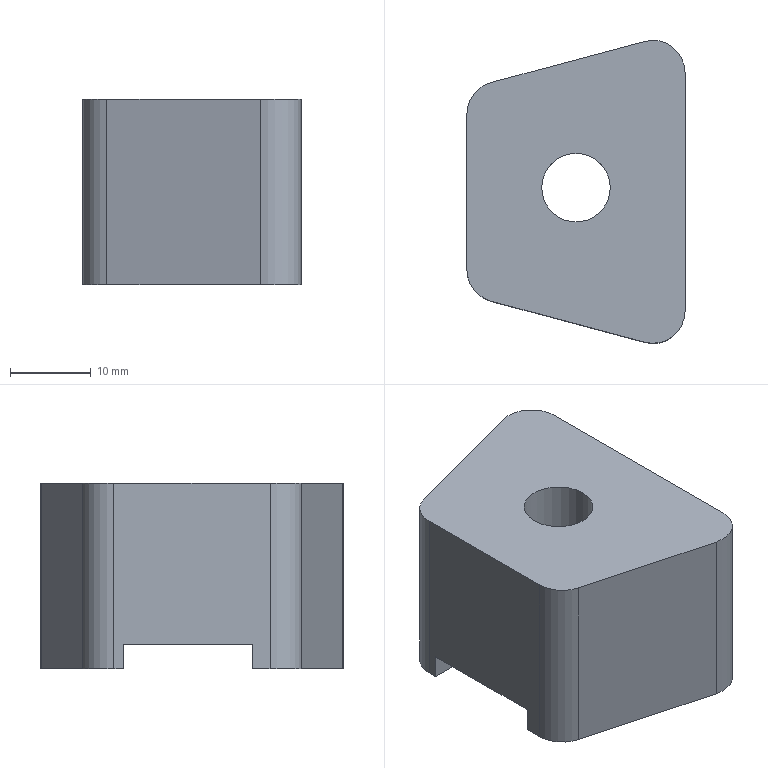Part | NX | features solid 2 | 1 solid | 17 faces | box 27 x 37.502 x 23 mm | volume 16532 mm3 | plane 11 | cylinder 6 | commonest cylinder face diameters 8 x4 8.5 x1 14 x1
STEP:
#1=CARTESIAN_POINT('',(1429.324,0.,20.));
#2=VERTEX_POINT('',#1);
#3=CARTESIAN_POINT('',(1425.074,0.,20.));
#4=DIRECTION('',(0.,0.,1.));
#5=DIRECTION('',(1.,0.,0.));
#6=AXIS2_PLACEMENT_3D('',#3,#4,#5);
#7=CIRCLE('',#6,4.25);
#8=EDGE_CURVE('',#2,#2,#7,.T.);
#9=ORIENTED_EDGE('',*,*,#8,.F.);
#10=EDGE_LOOP('',(#9));
#11=FACE_BOUND('',#10,.T.);
#12=CARTESIAN_POINT('',(1414.539,-14.041,20.));
#13=VERTEX_POINT('',#12);
#14=CARTESIAN_POINT('',(1433.539,-19.132,20.));
#15=VERTEX_POINT('',#14);
#16=CARTESIAN_POINT('',(1515.869,-41.192,20.));
#17=DIRECTION('',(0.9659,-0.2588,0.));
#18=VECTOR('',#17,1000.);
#19=LINE('',#16,#18);
#20=EDGE_CURVE('',#13,#15,#19,.T.);
#21=ORIENTED_EDGE('',*,*,#20,.T.);
#22=CARTESIAN_POINT('',(1438.574,-15.268,20.));
#23=VERTEX_POINT('',#22);
#24=CARTESIAN_POINT('',(1434.574,-15.268,20.));
#25=DIRECTION('',(0.,0.,1.));
#26=DIRECTION('',(1.,0.,0.));
#27=AXIS2_PLACEMENT_3D('',#24,#25,#26);
#28=CIRCLE('',#27,4.);
#29=EDGE_CURVE('',#15,#23,#28,.T.);
#30=ORIENTED_EDGE('',*,*,#29,.T.);
#31=CARTESIAN_POINT('',(1438.574,14.233,20.));
#32=VERTEX_POINT('',#31);
#33=CARTESIAN_POINT('',(1438.574,-11.19,20.));
#34=DIRECTION('',(0.,-1.,0.));
#35=VECTOR('',#34,1000.);
#36=LINE('',#33,#35);
#37=EDGE_CURVE('',#32,#23,#36,.T.);
#38=ORIENTED_EDGE('',*,*,#37,.F.);
#39=CARTESIAN_POINT('',(1433.539,18.097,20.));
#40=VERTEX_POINT('',#39);
#41=CARTESIAN_POINT('',(1434.574,14.233,20.));
#42=DIRECTION('',(0.,0.,1.));
#43=DIRECTION('',(1.,0.,0.));
#44=AXIS2_PLACEMENT_3D('',#41,#42,#43);
#45=CIRCLE('',#44,4.);
#46=EDGE_CURVE('',#32,#40,#45,.T.);
#47=ORIENTED_EDGE('',*,*,#46,.T.);
#48=CARTESIAN_POINT('',(1414.539,13.006,20.));
#49=VERTEX_POINT('',#48);
#50=CARTESIAN_POINT('',(1460.853,25.416,20.));
#51=DIRECTION('',(-0.9659,-0.2588,0.));
#52=VECTOR('',#51,1000.);
#53=LINE('',#50,#52);
#54=EDGE_CURVE('',#40,#49,#53,.T.);
#55=ORIENTED_EDGE('',*,*,#54,.T.);
#56=CARTESIAN_POINT('',(1411.574,9.142,20.));
#57=VERTEX_POINT('',#56);
#58=CARTESIAN_POINT('',(1415.574,9.142,20.));
#59=DIRECTION('',(0.,0.,1.));
#60=DIRECTION('',(1.,0.,0.));
#61=AXIS2_PLACEMENT_3D('',#58,#59,#60);
#62=CIRCLE('',#61,4.);
#63=EDGE_CURVE('',#49,#57,#62,.T.);
#64=ORIENTED_EDGE('',*,*,#63,.T.);
#65=CARTESIAN_POINT('',(1411.574,-10.177,20.));
#66=VERTEX_POINT('',#65);
#67=CARTESIAN_POINT('',(1411.574,-7.,20.));
#68=DIRECTION('',(0.,1.,0.));
#69=VECTOR('',#68,1000.);
#70=LINE('',#67,#69);
#71=EDGE_CURVE('',#66,#57,#70,.T.);
#72=ORIENTED_EDGE('',*,*,#71,.F.);
#73=CARTESIAN_POINT('',(1415.574,-10.177,20.));
#74=DIRECTION('',(0.,0.,1.));
#75=DIRECTION('',(1.,0.,0.));
#76=AXIS2_PLACEMENT_3D('',#73,#74,#75);
#77=CIRCLE('',#76,4.);
#78=EDGE_CURVE('',#66,#13,#77,.T.);
#79=ORIENTED_EDGE('',*,*,#78,.T.);
#80=EDGE_LOOP('',(#21,#30,#38,#47,#55,#64,#72,#79));
#81=FACE_BOUND('',#80,.T.);
#82=CARTESIAN_POINT('',(1497.285,-110.548,20.));
#83=DIRECTION('',(0.,0.,1.));
#84=DIRECTION('',(1.,0.,0.));
#85=AXIS2_PLACEMENT_3D('',#82,#83,#84);
#86=PLANE('',#85);
#87=ADVANCED_FACE('',(#11,#81),#86,.T.);
#88=CARTESIAN_POINT('',(1438.574,-8.,0.));
#89=VERTEX_POINT('',#88);
#90=CARTESIAN_POINT('',(1411.574,-8.,0.));
#91=VERTEX_POINT('',#90);
#92=CARTESIAN_POINT('',(1423.85,-8.,0.));
#93=DIRECTION('',(-1.,0.,0.));
#94=VECTOR('',#93,1000.);
#95=LINE('',#92,#94);
#96=EDGE_CURVE('',#89,#91,#95,.T.);
#97=ORIENTED_EDGE('',*,*,#96,.F.);
#98=CARTESIAN_POINT('',(1438.574,-8.,-3.));
#99=VERTEX_POINT('',#98);
#100=CARTESIAN_POINT('',(1438.574,-8.,-5.));
#101=DIRECTION('',(0.,0.,1.));
#102=VECTOR('',#101,1000.);
#103=LINE('',#100,#102);
#104=EDGE_CURVE('',#99,#89,#103,.T.);
#105=ORIENTED_EDGE('',*,*,#104,.F.);
#106=CARTESIAN_POINT('',(1411.574,-8.,-3.));
#107=VERTEX_POINT('',#106);
#108=CARTESIAN_POINT('',(268.879,-8.,-3.));
#109=DIRECTION('',(-1.,0.,0.));
#110=VECTOR('',#109,1000.);
#111=LINE('',#108,#110);
#112=EDGE_CURVE('',#107,#99,#111,.F.);
#113=ORIENTED_EDGE('',*,*,#112,.F.);
#114=CARTESIAN_POINT('',(1411.574,-8.,-5.));
#115=DIRECTION('',(0.,0.,1.));
#116=VECTOR('',#115,1000.);
#117=LINE('',#114,#116);
#118=EDGE_CURVE('',#107,#91,#117,.T.);
#119=ORIENTED_EDGE('',*,*,#118,.T.);
#120=EDGE_LOOP('',(#97,#105,#113,#119));
#121=FACE_BOUND('',#120,.T.);
#122=CARTESIAN_POINT('',(1423.85,-8.,-5.));
#123=DIRECTION('',(0.,1.,0.));
#124=DIRECTION('',(0.,0.,-1.));
#125=AXIS2_PLACEMENT_3D('',#122,#123,#124);
#126=PLANE('',#125);
#127=ADVANCED_FACE('',(#121),#126,.T.);
#128=CARTESIAN_POINT('',(1438.574,-15.268,-3.));
#129=VERTEX_POINT('',#128);
#130=CARTESIAN_POINT('',(1438.574,0.,-3.));
#131=DIRECTION('',(0.,1.,0.));
#132=VECTOR('',#131,1000.);
#133=LINE('',#130,#132);
#134=EDGE_CURVE('',#99,#129,#133,.F.);
#135=ORIENTED_EDGE('',*,*,#134,.T.);
#136=CARTESIAN_POINT('',(1433.539,-19.132,-3.));
#137=VERTEX_POINT('',#136);
#138=CARTESIAN_POINT('',(1434.574,-15.268,-3.));
#139=DIRECTION('',(0.,0.,1.));
#140=DIRECTION('',(1.,0.,0.));
#141=AXIS2_PLACEMENT_3D('',#138,#139,#140);
#142=CIRCLE('',#141,4.);
#143=EDGE_CURVE('',#129,#137,#142,.F.);
#144=ORIENTED_EDGE('',*,*,#143,.T.);
#145=CARTESIAN_POINT('',(1414.539,-14.041,-3.));
#146=VERTEX_POINT('',#145);
#147=CARTESIAN_POINT('',(1417.086,-14.724,-3.));
#148=DIRECTION('',(-0.9659,0.2588,0.));
#149=VECTOR('',#148,1000.);
#150=LINE('',#147,#149);
#151=EDGE_CURVE('',#146,#137,#150,.F.);
#152=ORIENTED_EDGE('',*,*,#151,.F.);
#153=CARTESIAN_POINT('',(1411.574,-10.177,-3.));
#154=VERTEX_POINT('',#153);
#155=CARTESIAN_POINT('',(1415.574,-10.177,-3.));
#156=DIRECTION('',(0.,0.,1.));
#157=DIRECTION('',(1.,0.,0.));
#158=AXIS2_PLACEMENT_3D('',#155,#156,#157);
#159=CIRCLE('',#158,4.);
#160=EDGE_CURVE('',#146,#154,#159,.F.);
#161=ORIENTED_EDGE('',*,*,#160,.T.);
#162=CARTESIAN_POINT('',(1411.574,0.,-3.));
#163=DIRECTION('',(0.,-1.,0.));
#164=VECTOR('',#163,1000.);
#165=LINE('',#162,#164);
#166=EDGE_CURVE('',#154,#107,#165,.F.);
#167=ORIENTED_EDGE('',*,*,#166,.T.);
#168=ORIENTED_EDGE('',*,*,#112,.T.);
#169=EDGE_LOOP('',(#135,#144,#152,#161,#167,#168));
#170=FACE_BOUND('',#169,.T.);
#171=CARTESIAN_POINT('',(268.879,0.,-3.));
#172=DIRECTION('',(0.,0.,1.));
#173=DIRECTION('',(1.,0.,0.));
#174=AXIS2_PLACEMENT_3D('',#171,#172,#173);
#175=PLANE('',#174);
#176=ADVANCED_FACE('',(#170),#175,.F.);
#177=ORIENTED_EDGE('',*,*,#151,.T.);
#178=CARTESIAN_POINT('',(1433.539,-19.132,-16.4));
#179=DIRECTION('',(0.,0.,-1.));
#180=VECTOR('',#179,1000.);
#181=LINE('',#178,#180);
#182=EDGE_CURVE('',#137,#15,#181,.F.);
#183=ORIENTED_EDGE('',*,*,#182,.T.);
#184=ORIENTED_EDGE('',*,*,#20,.F.);
#185=CARTESIAN_POINT('',(1414.539,-14.041,-16.4));
#186=DIRECTION('',(0.,0.,1.));
#187=VECTOR('',#186,1000.);
#188=LINE('',#185,#187);
#189=EDGE_CURVE('',#13,#146,#188,.F.);
#190=ORIENTED_EDGE('',*,*,#189,.T.);
#191=EDGE_LOOP('',(#177,#183,#184,#190));
#192=FACE_BOUND('',#191,.T.);
#193=CARTESIAN_POINT('',(1417.086,-14.724,-16.4));
#194=DIRECTION('',(-0.2588,-0.9659,0.));
#195=DIRECTION('',(-0.9659,0.2588,0.));
#196=AXIS2_PLACEMENT_3D('',#193,#194,#195);
#197=PLANE('',#196);
#198=ADVANCED_FACE('',(#192),#197,.T.);
#199=ORIENTED_EDGE('',*,*,#37,.T.);
#200=CARTESIAN_POINT('',(1438.574,-15.268,-5.));
#201=DIRECTION('',(0.,0.,-1.));
#202=VECTOR('',#201,1000.);
#203=LINE('',#200,#202);
#204=EDGE_CURVE('',#23,#129,#203,.T.);
#205=ORIENTED_EDGE('',*,*,#204,.T.);
#206=ORIENTED_EDGE('',*,*,#134,.F.);
#207=ORIENTED_EDGE('',*,*,#104,.T.);
#208=CARTESIAN_POINT('',(1438.574,8.,0.));
#209=VERTEX_POINT('',#208);
#210=CARTESIAN_POINT('',(1438.574,1232.968,0.));
#211=DIRECTION('',(0.,-1.,0.));
#212=VECTOR('',#211,1000.);
#213=LINE('',#210,#212);
#214=EDGE_CURVE('',#209,#89,#213,.T.);
#215=ORIENTED_EDGE('',*,*,#214,.F.);
#216=CARTESIAN_POINT('',(1438.574,8.,-3.));
#217=VERTEX_POINT('',#216);
#218=CARTESIAN_POINT('',(1438.574,8.,-5.));
#219=DIRECTION('',(0.,0.,1.));
#220=VECTOR('',#219,1000.);
#221=LINE('',#218,#220);
#222=EDGE_CURVE('',#217,#209,#221,.T.);
#223=ORIENTED_EDGE('',*,*,#222,.F.);
#224=CARTESIAN_POINT('',(1438.574,14.233,-3.));
#225=VERTEX_POINT('',#224);
#226=CARTESIAN_POINT('',(1438.574,-11.19,-3.));
#227=DIRECTION('',(0.,-1.,0.));
#228=VECTOR('',#227,1000.);
#229=LINE('',#226,#228);
#230=EDGE_CURVE('',#217,#225,#229,.F.);
#231=ORIENTED_EDGE('',*,*,#230,.T.);
#232=CARTESIAN_POINT('',(1438.574,14.233,-5.));
#233=DIRECTION('',(0.,0.,1.));
#234=VECTOR('',#233,1000.);
#235=LINE('',#232,#234);
#236=EDGE_CURVE('',#225,#32,#235,.T.);
#237=ORIENTED_EDGE('',*,*,#236,.T.);
#238=EDGE_LOOP('',(#199,#205,#206,#207,#215,#223,#231,#237));
#239=FACE_BOUND('',#238,.T.);
#240=CARTESIAN_POINT('',(1438.574,-11.19,-5.));
#241=DIRECTION('',(1.,0.,0.));
#242=DIRECTION('',(0.,0.,-1.));
#243=AXIS2_PLACEMENT_3D('',#240,#241,#242);
#244=PLANE('',#243);
#245=ADVANCED_FACE('',(#239),#244,.T.);
#246=ORIENTED_EDGE('',*,*,#166,.F.);
#247=CARTESIAN_POINT('',(1411.574,-10.177,-5.));
#248=DIRECTION('',(0.,0.,1.));
#249=VECTOR('',#248,1000.);
#250=LINE('',#247,#249);
#251=EDGE_CURVE('',#154,#66,#250,.T.);
#252=ORIENTED_EDGE('',*,*,#251,.T.);
#253=ORIENTED_EDGE('',*,*,#71,.T.);
#254=CARTESIAN_POINT('',(1411.574,9.142,-3.));
#255=VERTEX_POINT('',#254);
#256=CARTESIAN_POINT('',(1411.574,9.142,-5.));
#257=DIRECTION('',(0.,0.,-1.));
#258=VECTOR('',#257,1000.);
#259=LINE('',#256,#258);
#260=EDGE_CURVE('',#57,#255,#259,.T.);
#261=ORIENTED_EDGE('',*,*,#260,.T.);
#262=CARTESIAN_POINT('',(1411.574,8.,-3.));
#263=VERTEX_POINT('',#262);
#264=CARTESIAN_POINT('',(1411.574,0.,-3.));
#265=DIRECTION('',(0.,-1.,0.));
#266=VECTOR('',#265,1000.);
#267=LINE('',#264,#266);
#268=EDGE_CURVE('',#263,#255,#267,.F.);
#269=ORIENTED_EDGE('',*,*,#268,.F.);
#270=CARTESIAN_POINT('',(1411.574,8.,0.));
#271=VERTEX_POINT('',#270);
#272=CARTESIAN_POINT('',(1411.574,8.,-5.));
#273=DIRECTION('',(0.,0.,-1.));
#274=VECTOR('',#273,1000.);
#275=LINE('',#272,#274);
#276=EDGE_CURVE('',#271,#263,#275,.T.);
#277=ORIENTED_EDGE('',*,*,#276,.F.);
#278=CARTESIAN_POINT('',(1411.574,1232.968,0.));
#279=DIRECTION('',(0.,1.,0.));
#280=VECTOR('',#279,1000.);
#281=LINE('',#278,#280);
#282=EDGE_CURVE('',#91,#271,#281,.T.);
#283=ORIENTED_EDGE('',*,*,#282,.F.);
#284=ORIENTED_EDGE('',*,*,#118,.F.);
#285=EDGE_LOOP('',(#246,#252,#253,#261,#269,#277,#283,#284));
#286=FACE_BOUND('',#285,.T.);
#287=CARTESIAN_POINT('',(1411.574,-7.,-5.));
#288=DIRECTION('',(-1.,0.,0.));
#289=DIRECTION('',(0.,0.,1.));
#290=AXIS2_PLACEMENT_3D('',#287,#288,#289);
#291=PLANE('',#290);
#292=ADVANCED_FACE('',(#286),#291,.T.);
#293=CARTESIAN_POINT('',(1423.85,8.,0.));
#294=DIRECTION('',(1.,0.,0.));
#295=VECTOR('',#294,1000.);
#296=LINE('',#293,#295);
#297=EDGE_CURVE('',#271,#209,#296,.T.);
#298=ORIENTED_EDGE('',*,*,#297,.F.);
#299=ORIENTED_EDGE('',*,*,#276,.T.);
#300=CARTESIAN_POINT('',(1423.85,8.,-3.));
#301=DIRECTION('',(-1.,0.,0.));
#302=VECTOR('',#301,1000.);
#303=LINE('',#300,#302);
#304=EDGE_CURVE('',#263,#217,#303,.F.);
#305=ORIENTED_EDGE('',*,*,#304,.T.);
#306=ORIENTED_EDGE('',*,*,#222,.T.);
#307=EDGE_LOOP('',(#298,#299,#305,#306));
#308=FACE_BOUND('',#307,.T.);
#309=CARTESIAN_POINT('',(1423.85,8.,-5.));
#310=DIRECTION('',(0.,-1.,0.));
#311=DIRECTION('',(0.,0.,-1.));
#312=AXIS2_PLACEMENT_3D('',#309,#310,#311);
#313=PLANE('',#312);
#314=ADVANCED_FACE('',(#308),#313,.T.);
#315=CARTESIAN_POINT('',(1414.539,13.006,-3.));
#316=VERTEX_POINT('',#315);
#317=CARTESIAN_POINT('',(1433.539,18.097,-3.));
#318=VERTEX_POINT('',#317);
#319=CARTESIAN_POINT('',(342.372,-274.28,-3.));
#320=DIRECTION('',(-0.9659,-0.2588,0.));
#321=VECTOR('',#320,1000.);
#322=LINE('',#319,#321);
#323=EDGE_CURVE('',#316,#318,#322,.F.);
#324=ORIENTED_EDGE('',*,*,#323,.T.);
#325=CARTESIAN_POINT('',(1434.574,14.233,-3.));
#326=DIRECTION('',(0.,0.,1.));
#327=DIRECTION('',(1.,0.,0.));
#328=AXIS2_PLACEMENT_3D('',#325,#326,#327);
#329=CIRCLE('',#328,4.);
#330=EDGE_CURVE('',#318,#225,#329,.F.);
#331=ORIENTED_EDGE('',*,*,#330,.T.);
#332=ORIENTED_EDGE('',*,*,#230,.F.);
#333=ORIENTED_EDGE('',*,*,#304,.F.);
#334=ORIENTED_EDGE('',*,*,#268,.T.);
#335=CARTESIAN_POINT('',(1415.574,9.142,-3.));
#336=DIRECTION('',(0.,0.,1.));
#337=DIRECTION('',(1.,0.,0.));
#338=AXIS2_PLACEMENT_3D('',#335,#336,#337);
#339=CIRCLE('',#338,4.);
#340=EDGE_CURVE('',#255,#316,#339,.F.);
#341=ORIENTED_EDGE('',*,*,#340,.T.);
#342=EDGE_LOOP('',(#324,#331,#332,#333,#334,#341));
#343=FACE_BOUND('',#342,.T.);
#344=CARTESIAN_POINT('',(268.879,0.,-3.));
#345=DIRECTION('',(0.,0.,1.));
#346=DIRECTION('',(1.,0.,0.));
#347=AXIS2_PLACEMENT_3D('',#344,#345,#346);
#348=PLANE('',#347);
#349=ADVANCED_FACE('',(#343),#348,.F.);
#350=ORIENTED_EDGE('',*,*,#54,.F.);
#351=CARTESIAN_POINT('',(1433.539,18.097,-16.4));
#352=DIRECTION('',(0.,0.,1.));
#353=VECTOR('',#352,1000.);
#354=LINE('',#351,#353);
#355=EDGE_CURVE('',#40,#318,#354,.F.);
#356=ORIENTED_EDGE('',*,*,#355,.T.);
#357=ORIENTED_EDGE('',*,*,#323,.F.);
#358=CARTESIAN_POINT('',(1414.539,13.006,-16.4));
#359=DIRECTION('',(0.,0.,-1.));
#360=VECTOR('',#359,1000.);
#361=LINE('',#358,#360);
#362=EDGE_CURVE('',#316,#49,#361,.F.);
#363=ORIENTED_EDGE('',*,*,#362,.T.);
#364=EDGE_LOOP('',(#350,#356,#357,#363));
#365=FACE_BOUND('',#364,.T.);
#366=CARTESIAN_POINT('',(1417.345,13.758,-16.4));
#367=DIRECTION('',(-0.2588,0.9659,0.));
#368=DIRECTION('',(-0.9659,-0.2588,0.));
#369=AXIS2_PLACEMENT_3D('',#366,#367,#368);
#370=PLANE('',#369);
#371=ADVANCED_FACE('',(#365),#370,.T.);
#372=ORIENTED_EDGE('',*,*,#297,.T.);
#373=ORIENTED_EDGE('',*,*,#214,.T.);
#374=ORIENTED_EDGE('',*,*,#96,.T.);
#375=ORIENTED_EDGE('',*,*,#282,.T.);
#376=EDGE_LOOP('',(#372,#373,#374,#375));
#377=FACE_BOUND('',#376,.T.);
#378=CARTESIAN_POINT('',(1418.074,0.,0.));
#379=VERTEX_POINT('',#378);
#380=CARTESIAN_POINT('',(1425.074,0.,0.));
#381=DIRECTION('',(0.,0.,-1.));
#382=DIRECTION('',(-1.,0.,0.));
#383=AXIS2_PLACEMENT_3D('',#380,#381,#382);
#384=CIRCLE('',#383,7.);
#385=EDGE_CURVE('',#379,#379,#384,.F.);
#386=ORIENTED_EDGE('',*,*,#385,.T.);
#387=EDGE_LOOP('',(#386));
#388=FACE_BOUND('',#387,.T.);
#389=CARTESIAN_POINT('',(476.557,1232.968,0.));
#390=DIRECTION('',(0.,0.,-1.));
#391=DIRECTION('',(-0.9659,0.2588,0.));
#392=AXIS2_PLACEMENT_3D('',#389,#390,#391);
#393=PLANE('',#392);
#394=ADVANCED_FACE('',(#377,#388),#393,.T.);
#395=ORIENTED_EDGE('',*,*,#78,.F.);
#396=ORIENTED_EDGE('',*,*,#251,.F.);
#397=ORIENTED_EDGE('',*,*,#160,.F.);
#398=ORIENTED_EDGE('',*,*,#189,.F.);
#399=EDGE_LOOP('',(#395,#396,#397,#398));
#400=FACE_BOUND('',#399,.T.);
#401=CARTESIAN_POINT('',(1415.574,-10.177,-5.));
#402=DIRECTION('',(0.,0.,1.));
#403=DIRECTION('',(1.,0.,0.));
#404=AXIS2_PLACEMENT_3D('',#401,#402,#403);
#405=CYLINDRICAL_SURFACE('',#404,4.);
#406=ADVANCED_FACE('',(#400),#405,.T.);
#407=ORIENTED_EDGE('',*,*,#340,.F.);
#408=ORIENTED_EDGE('',*,*,#260,.F.);
#409=ORIENTED_EDGE('',*,*,#63,.F.);
#410=ORIENTED_EDGE('',*,*,#362,.F.);
#411=EDGE_LOOP('',(#407,#408,#409,#410));
#412=FACE_BOUND('',#411,.T.);
#413=CARTESIAN_POINT('',(1415.574,9.142,-5.));
#414=DIRECTION('',(0.,0.,-1.));
#415=DIRECTION('',(-1.,0.,0.));
#416=AXIS2_PLACEMENT_3D('',#413,#414,#415);
#417=CYLINDRICAL_SURFACE('',#416,4.);
#418=ADVANCED_FACE('',(#412),#417,.T.);
#419=ORIENTED_EDGE('',*,*,#8,.T.);
#420=EDGE_LOOP('',(#419));
#421=FACE_BOUND('',#420,.T.);
#422=CARTESIAN_POINT('',(1429.324,0.,10.));
#423=VERTEX_POINT('',#422);
#424=CARTESIAN_POINT('',(1425.074,0.,10.));
#425=DIRECTION('',(0.,0.,1.));
#426=DIRECTION('',(1.,0.,0.));
#427=AXIS2_PLACEMENT_3D('',#424,#425,#426);
#428=CIRCLE('',#427,4.25);
#429=EDGE_CURVE('',#423,#423,#428,.F.);
#430=ORIENTED_EDGE('',*,*,#429,.T.);
#431=EDGE_LOOP('',(#430));
#432=FACE_BOUND('',#431,.T.);
#433=CARTESIAN_POINT('',(1425.074,0.,50.));
#434=DIRECTION('',(0.,0.,1.));
#435=DIRECTION('',(1.,0.,0.));
#436=AXIS2_PLACEMENT_3D('',#433,#434,#435);
#437=CYLINDRICAL_SURFACE('',#436,4.25);
#438=ADVANCED_FACE('',(#421,#432),#437,.F.);
#439=ORIENTED_EDGE('',*,*,#429,.F.);
#440=EDGE_LOOP('',(#439));
#441=FACE_BOUND('',#440,.T.);
#442=CARTESIAN_POINT('',(1432.074,0.,10.));
#443=VERTEX_POINT('',#442);
#444=CARTESIAN_POINT('',(1425.074,0.,10.));
#445=DIRECTION('',(0.,0.,1.));
#446=DIRECTION('',(1.,0.,0.));
#447=AXIS2_PLACEMENT_3D('',#444,#445,#446);
#448=CIRCLE('',#447,7.);
#449=EDGE_CURVE('',#443,#443,#448,.F.);
#450=ORIENTED_EDGE('',*,*,#449,.T.);
#451=EDGE_LOOP('',(#450));
#452=FACE_BOUND('',#451,.T.);
#453=CARTESIAN_POINT('',(1425.074,0.,10.));
#454=DIRECTION('',(0.,0.,1.));
#455=DIRECTION('',(1.,0.,0.));
#456=AXIS2_PLACEMENT_3D('',#453,#454,#455);
#457=PLANE('',#456);
#458=ADVANCED_FACE('',(#441,#452),#457,.F.);
#459=ORIENTED_EDGE('',*,*,#449,.F.);
#460=EDGE_LOOP('',(#459));
#461=FACE_BOUND('',#460,.T.);
#462=ORIENTED_EDGE('',*,*,#385,.F.);
#463=EDGE_LOOP('',(#462));
#464=FACE_BOUND('',#463,.T.);
#465=CARTESIAN_POINT('',(1425.074,0.,0.));
#466=DIRECTION('',(0.,0.,1.));
#467=DIRECTION('',(1.,0.,0.));
#468=AXIS2_PLACEMENT_3D('',#465,#466,#467);
#469=CYLINDRICAL_SURFACE('',#468,7.);
#470=ADVANCED_FACE('',(#461,#464),#469,.F.);
#471=ORIENTED_EDGE('',*,*,#29,.F.);
#472=ORIENTED_EDGE('',*,*,#182,.F.);
#473=ORIENTED_EDGE('',*,*,#143,.F.);
#474=ORIENTED_EDGE('',*,*,#204,.F.);
#475=EDGE_LOOP('',(#471,#472,#473,#474));
#476=FACE_BOUND('',#475,.T.);
#477=CARTESIAN_POINT('',(1434.574,-15.268,-5.));
#478=DIRECTION('',(0.,0.,-1.));
#479=DIRECTION('',(-1.,0.,0.));
#480=AXIS2_PLACEMENT_3D('',#477,#478,#479);
#481=CYLINDRICAL_SURFACE('',#480,4.);
#482=ADVANCED_FACE('',(#476),#481,.T.);
#483=ORIENTED_EDGE('',*,*,#330,.F.);
#484=ORIENTED_EDGE('',*,*,#355,.F.);
#485=ORIENTED_EDGE('',*,*,#46,.F.);
#486=ORIENTED_EDGE('',*,*,#236,.F.);
#487=EDGE_LOOP('',(#483,#484,#485,#486));
#488=FACE_BOUND('',#487,.T.);
#489=CARTESIAN_POINT('',(1434.574,14.233,-5.));
#490=DIRECTION('',(0.,0.,1.));
#491=DIRECTION('',(1.,0.,0.));
#492=AXIS2_PLACEMENT_3D('',#489,#490,#491);
#493=CYLINDRICAL_SURFACE('',#492,4.);
#494=ADVANCED_FACE('',(#488),#493,.T.);
#495=CLOSED_SHELL('',(#87,#127,#176,#198,#245,#292,#314,#349,#371,#394,#406,#418,#438,#458,#470,#482,#494));
#496=MANIFOLD_SOLID_BREP('',#495);
#497=(LENGTH_UNIT()NAMED_UNIT(*)SI_UNIT(.MILLI.,.METRE.));
#498=UNCERTAINTY_MEASURE_WITH_UNIT(LENGTH_MEASURE(0.00001),#497,'','');
#499=(NAMED_UNIT(*)PLANE_ANGLE_UNIT()SI_UNIT($,.RADIAN.));
#500=(NAMED_UNIT(*)SI_UNIT($,.STERADIAN.)SOLID_ANGLE_UNIT());
#501=(GEOMETRIC_REPRESENTATION_CONTEXT(3)GLOBAL_UNCERTAINTY_ASSIGNED_CONTEXT((#498))GLOBAL_UNIT_ASSIGNED_CONTEXT((#497,#499,#500))REPRESENTATION_CONTEXT('',''));
#502=ADVANCED_BREP_SHAPE_REPRESENTATION('',(#496),#501);